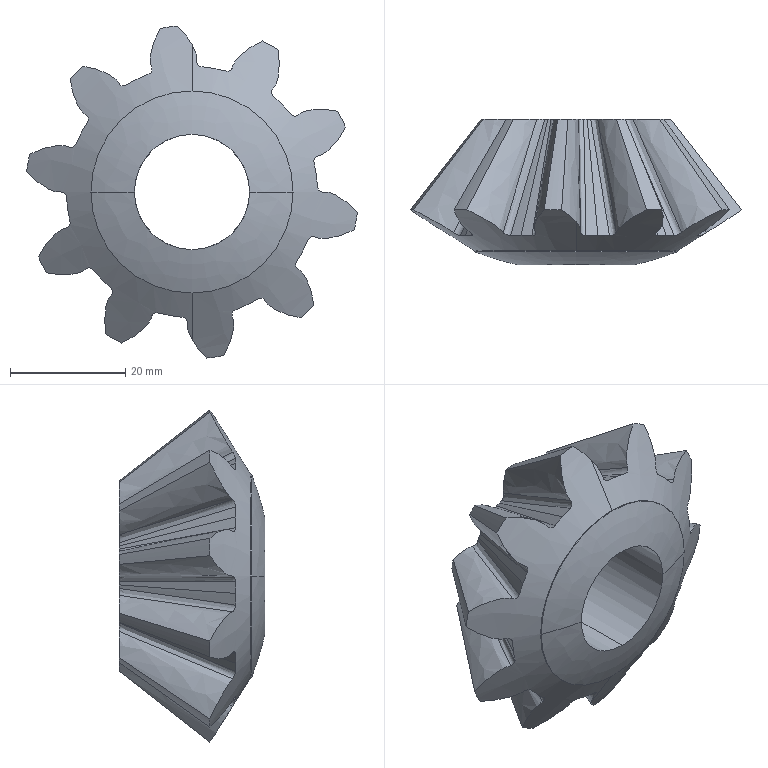Part | SolidWorks | features BaseBody 1 | 1 solid | 79 faces | box 57.348 x 25.263 x 57.563 mm | volume 22124 mm3 | spline 62 | cone 12 | cylinder 4 | plane 1 | commonest cylinder face diameters 20 x2 35.058 x2